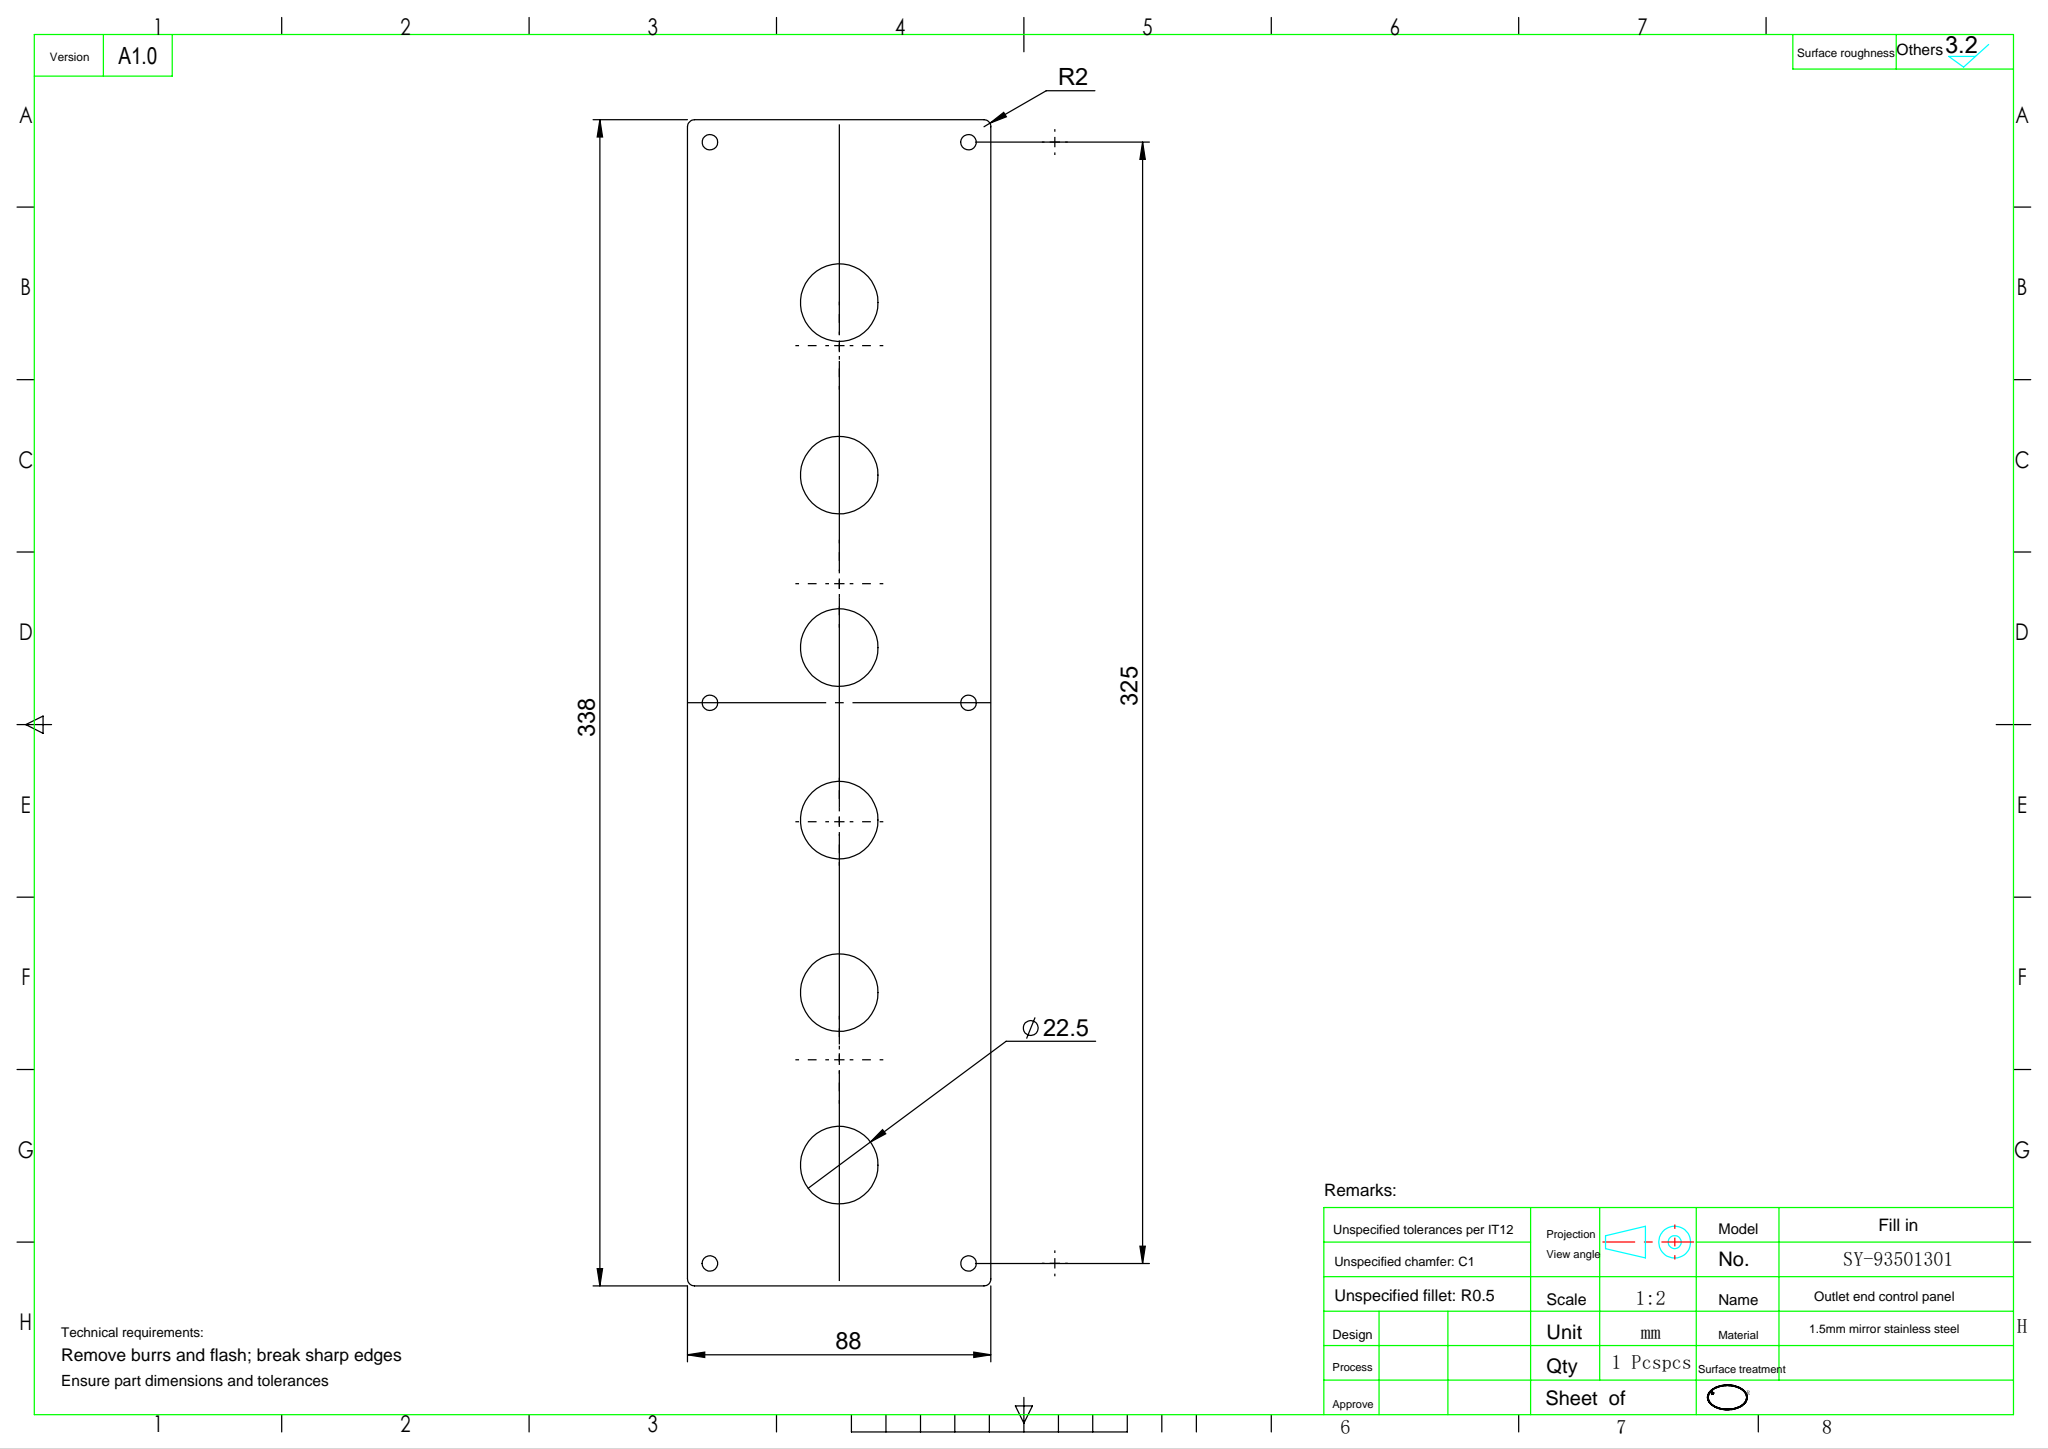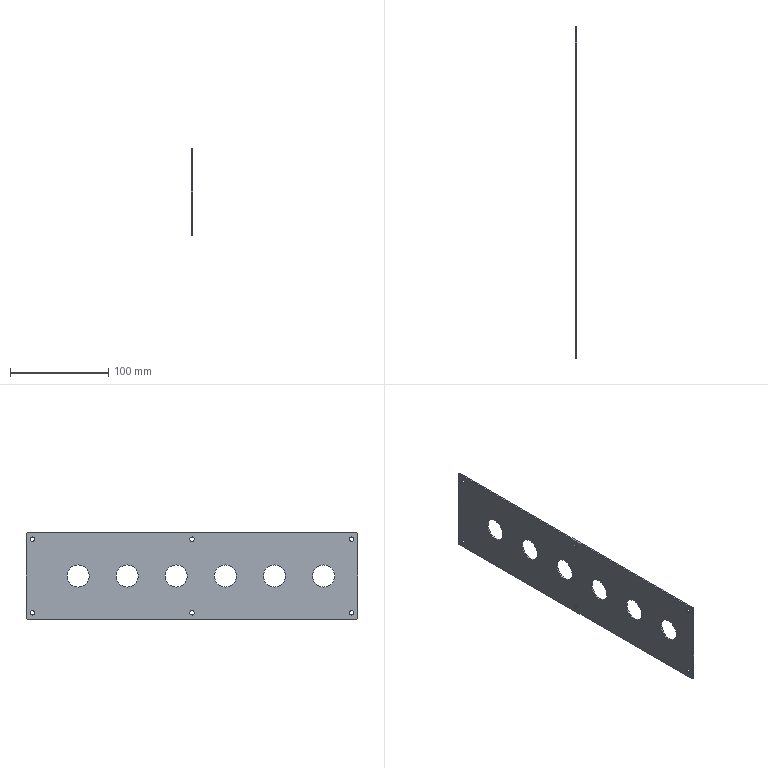Part | SolidWorks | features ICE 2, Fillet 1, FlatPattern 1, SMBaseFlange 1, SheetMetal 1 | 1 solid | 34 faces | box 1.5 x 338 x 88 mm | volume 40889 mm3 | cylinder 28 | plane 6 | commonest cylinder face diameters 4.5 x12 22.5 x12 4 x4